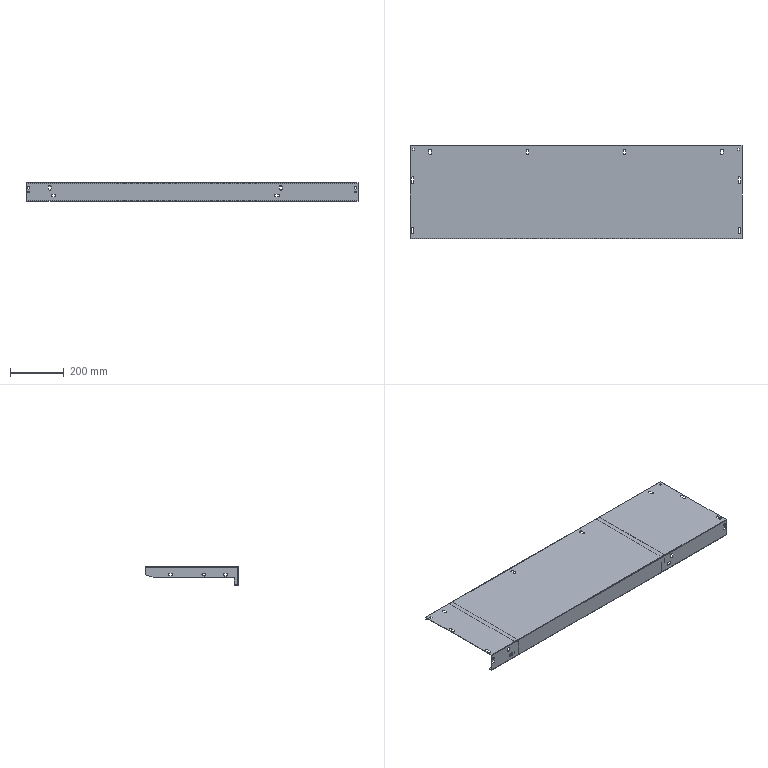Part | 3 solids | 218 faces | box 1240 x 349.5 x 70 mm | volume 903973 mm3 | plane 154 | cylinder 64 | commonest cylinder face diameters 10 x24 9 x12 11 x10 2 x4 6 x4 8 x4